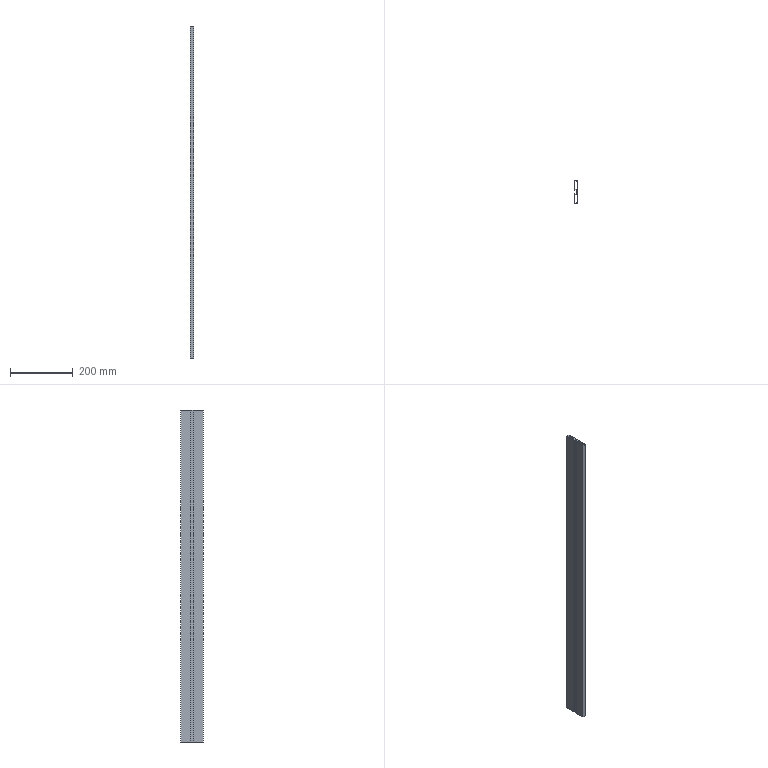Part | 1 solid | 22 faces | box 12 x 73 x 1060 mm | volume 385840 mm3 | plane 22
STEP:
#1=CARTESIAN_POINT('',(-12.,36.5,530.));
#2=VERTEX_POINT('',#1);
#3=CARTESIAN_POINT('',(-12.,4.5,530.));
#4=VERTEX_POINT('',#3);
#5=CARTESIAN_POINT('',(-12.,36.5,530.));
#6=DIRECTION('',(0.,-1.,0.));
#7=VECTOR('',#6,1000.);
#8=LINE('',#5,#7);
#9=EDGE_CURVE('',#2,#4,#8,.T.);
#10=ORIENTED_EDGE('',*,*,#9,.T.);
#11=CARTESIAN_POINT('',(-10.,4.5,530.));
#12=VERTEX_POINT('',#11);
#13=CARTESIAN_POINT('',(-12.,4.5,530.));
#14=DIRECTION('',(1.,0.,0.));
#15=VECTOR('',#14,1000.);
#16=LINE('',#13,#15);
#17=EDGE_CURVE('',#4,#12,#16,.T.);
#18=ORIENTED_EDGE('',*,*,#17,.T.);
#19=CARTESIAN_POINT('',(-10.,6.5,530.));
#20=VERTEX_POINT('',#19);
#21=CARTESIAN_POINT('',(-10.,4.5,530.));
#22=DIRECTION('',(0.,1.,0.));
#23=VECTOR('',#22,1000.);
#24=LINE('',#21,#23);
#25=EDGE_CURVE('',#12,#20,#24,.T.);
#26=ORIENTED_EDGE('',*,*,#25,.T.);
#27=CARTESIAN_POINT('',(-4.,6.5,530.));
#28=VERTEX_POINT('',#27);
#29=CARTESIAN_POINT('',(-10.,6.5,530.));
#30=DIRECTION('',(1.,0.,0.));
#31=VECTOR('',#30,1000.);
#32=LINE('',#29,#31);
#33=EDGE_CURVE('',#20,#28,#32,.T.);
#34=ORIENTED_EDGE('',*,*,#33,.T.);
#35=CARTESIAN_POINT('',(-4.,-6.5,530.));
#36=VERTEX_POINT('',#35);
#37=CARTESIAN_POINT('',(-4.,6.5,530.));
#38=DIRECTION('',(0.,-1.,0.));
#39=VECTOR('',#38,1000.);
#40=LINE('',#37,#39);
#41=EDGE_CURVE('',#28,#36,#40,.T.);
#42=ORIENTED_EDGE('',*,*,#41,.T.);
#43=CARTESIAN_POINT('',(-10.,-6.5,530.));
#44=VERTEX_POINT('',#43);
#45=CARTESIAN_POINT('',(-4.,-6.5,530.));
#46=DIRECTION('',(-1.,0.,0.));
#47=VECTOR('',#46,1000.);
#48=LINE('',#45,#47);
#49=EDGE_CURVE('',#36,#44,#48,.T.);
#50=ORIENTED_EDGE('',*,*,#49,.T.);
#51=CARTESIAN_POINT('',(-10.,-4.5,530.));
#52=VERTEX_POINT('',#51);
#53=CARTESIAN_POINT('',(-10.,-6.5,530.));
#54=DIRECTION('',(0.,1.,0.));
#55=VECTOR('',#54,1000.);
#56=LINE('',#53,#55);
#57=EDGE_CURVE('',#44,#52,#56,.T.);
#58=ORIENTED_EDGE('',*,*,#57,.T.);
#59=CARTESIAN_POINT('',(-12.,-4.5,530.));
#60=VERTEX_POINT('',#59);
#61=CARTESIAN_POINT('',(-10.,-4.5,530.));
#62=DIRECTION('',(-1.,0.,0.));
#63=VECTOR('',#62,1000.);
#64=LINE('',#61,#63);
#65=EDGE_CURVE('',#52,#60,#64,.T.);
#66=ORIENTED_EDGE('',*,*,#65,.T.);
#67=CARTESIAN_POINT('',(-12.,-36.5,530.));
#68=VERTEX_POINT('',#67);
#69=CARTESIAN_POINT('',(-12.,-4.5,530.));
#70=DIRECTION('',(0.,-1.,0.));
#71=VECTOR('',#70,1000.);
#72=LINE('',#69,#71);
#73=EDGE_CURVE('',#60,#68,#72,.T.);
#74=ORIENTED_EDGE('',*,*,#73,.T.);
#75=CARTESIAN_POINT('',(0.,-36.5,530.));
#76=VERTEX_POINT('',#75);
#77=CARTESIAN_POINT('',(-12.,-36.5,530.));
#78=DIRECTION('',(1.,0.,0.));
#79=VECTOR('',#78,1000.);
#80=LINE('',#77,#79);
#81=EDGE_CURVE('',#68,#76,#80,.T.);
#82=ORIENTED_EDGE('',*,*,#81,.T.);
#83=CARTESIAN_POINT('',(0.,36.5,530.));
#84=VERTEX_POINT('',#83);
#85=CARTESIAN_POINT('',(0.,-36.5,530.));
#86=DIRECTION('',(0.,1.,0.));
#87=VECTOR('',#86,1000.);
#88=LINE('',#85,#87);
#89=EDGE_CURVE('',#76,#84,#88,.T.);
#90=ORIENTED_EDGE('',*,*,#89,.T.);
#91=CARTESIAN_POINT('',(0.,36.5,530.));
#92=DIRECTION('',(-1.,0.,0.));
#93=VECTOR('',#92,1000.);
#94=LINE('',#91,#93);
#95=EDGE_CURVE('',#84,#2,#94,.T.);
#96=ORIENTED_EDGE('',*,*,#95,.T.);
#97=EDGE_LOOP('',(#10,#18,#26,#34,#42,#50,#58,#66,#74,#82,#90,#96));
#98=FACE_OUTER_BOUND('',#97,.T.);
#99=CARTESIAN_POINT('',(-10.,-34.5,530.));
#100=VERTEX_POINT('',#99);
#101=CARTESIAN_POINT('',(-2.,-34.5,530.));
#102=VERTEX_POINT('',#101);
#103=CARTESIAN_POINT('',(-2.,-34.5,530.));
#104=DIRECTION('',(1.,0.,0.));
#105=VECTOR('',#104,1000.);
#106=LINE('',#103,#105);
#107=EDGE_CURVE('',#100,#102,#106,.T.);
#108=ORIENTED_EDGE('',*,*,#107,.F.);
#109=CARTESIAN_POINT('',(-10.,-8.5,530.));
#110=VERTEX_POINT('',#109);
#111=CARTESIAN_POINT('',(-10.,-34.5,530.));
#112=DIRECTION('',(0.,-1.,0.));
#113=VECTOR('',#112,1000.);
#114=LINE('',#111,#113);
#115=EDGE_CURVE('',#110,#100,#114,.T.);
#116=ORIENTED_EDGE('',*,*,#115,.F.);
#117=CARTESIAN_POINT('',(-2.,-8.5,530.));
#118=VERTEX_POINT('',#117);
#119=CARTESIAN_POINT('',(-10.,-8.5,530.));
#120=DIRECTION('',(-1.,0.,0.));
#121=VECTOR('',#120,1000.);
#122=LINE('',#119,#121);
#123=EDGE_CURVE('',#118,#110,#122,.T.);
#124=ORIENTED_EDGE('',*,*,#123,.F.);
#125=CARTESIAN_POINT('',(-2.,-8.5,530.));
#126=DIRECTION('',(0.,1.,0.));
#127=VECTOR('',#126,1000.);
#128=LINE('',#125,#127);
#129=EDGE_CURVE('',#102,#118,#128,.T.);
#130=ORIENTED_EDGE('',*,*,#129,.F.);
#131=EDGE_LOOP('',(#108,#116,#124,#130));
#132=FACE_BOUND('',#131,.T.);
#133=CARTESIAN_POINT('',(-10.,34.5,530.));
#134=VERTEX_POINT('',#133);
#135=CARTESIAN_POINT('',(-10.,8.5,530.));
#136=VERTEX_POINT('',#135);
#137=CARTESIAN_POINT('',(-10.,8.5,530.));
#138=DIRECTION('',(0.,-1.,0.));
#139=VECTOR('',#138,1000.);
#140=LINE('',#137,#139);
#141=EDGE_CURVE('',#134,#136,#140,.T.);
#142=ORIENTED_EDGE('',*,*,#141,.F.);
#143=CARTESIAN_POINT('',(-2.,34.5,530.));
#144=VERTEX_POINT('',#143);
#145=CARTESIAN_POINT('',(-10.,34.5,530.));
#146=DIRECTION('',(-1.,0.,0.));
#147=VECTOR('',#146,1000.);
#148=LINE('',#145,#147);
#149=EDGE_CURVE('',#144,#134,#148,.T.);
#150=ORIENTED_EDGE('',*,*,#149,.F.);
#151=CARTESIAN_POINT('',(-2.,8.5,530.));
#152=VERTEX_POINT('',#151);
#153=CARTESIAN_POINT('',(-2.,34.5,530.));
#154=DIRECTION('',(0.,1.,0.));
#155=VECTOR('',#154,1000.);
#156=LINE('',#153,#155);
#157=EDGE_CURVE('',#152,#144,#156,.T.);
#158=ORIENTED_EDGE('',*,*,#157,.F.);
#159=CARTESIAN_POINT('',(-2.,8.5,530.));
#160=DIRECTION('',(1.,0.,0.));
#161=VECTOR('',#160,1000.);
#162=LINE('',#159,#161);
#163=EDGE_CURVE('',#136,#152,#162,.T.);
#164=ORIENTED_EDGE('',*,*,#163,.F.);
#165=EDGE_LOOP('',(#142,#150,#158,#164));
#166=FACE_BOUND('',#165,.T.);
#167=CARTESIAN_POINT('',(0.,0.,530.));
#168=DIRECTION('',(0.,0.,1.));
#169=DIRECTION('',(1.,0.,0.));
#170=AXIS2_PLACEMENT_3D('',#167,#168,#169);
#171=PLANE('',#170);
#172=ADVANCED_FACE('',(#98,#132,#166),#171,.T.);
#173=CARTESIAN_POINT('',(-10.,-8.5,-530.));
#174=VERTEX_POINT('',#173);
#175=CARTESIAN_POINT('',(-10.,-34.5,-530.));
#176=VERTEX_POINT('',#175);
#177=CARTESIAN_POINT('',(-10.,-34.5,-530.));
#178=DIRECTION('',(0.,-1.,0.));
#179=VECTOR('',#178,1000.);
#180=LINE('',#177,#179);
#181=EDGE_CURVE('',#174,#176,#180,.T.);
#182=ORIENTED_EDGE('',*,*,#181,.T.);
#183=CARTESIAN_POINT('',(-2.,-34.5,-530.));
#184=VERTEX_POINT('',#183);
#185=CARTESIAN_POINT('',(-2.,-34.5,-530.));
#186=DIRECTION('',(1.,0.,0.));
#187=VECTOR('',#186,1000.);
#188=LINE('',#185,#187);
#189=EDGE_CURVE('',#176,#184,#188,.T.);
#190=ORIENTED_EDGE('',*,*,#189,.T.);
#191=CARTESIAN_POINT('',(-2.,-8.5,-530.));
#192=VERTEX_POINT('',#191);
#193=CARTESIAN_POINT('',(-2.,-8.5,-530.));
#194=DIRECTION('',(0.,1.,0.));
#195=VECTOR('',#194,1000.);
#196=LINE('',#193,#195);
#197=EDGE_CURVE('',#184,#192,#196,.T.);
#198=ORIENTED_EDGE('',*,*,#197,.T.);
#199=CARTESIAN_POINT('',(-10.,-8.5,-530.));
#200=DIRECTION('',(-1.,0.,0.));
#201=VECTOR('',#200,1000.);
#202=LINE('',#199,#201);
#203=EDGE_CURVE('',#192,#174,#202,.T.);
#204=ORIENTED_EDGE('',*,*,#203,.T.);
#205=EDGE_LOOP('',(#182,#190,#198,#204));
#206=FACE_BOUND('',#205,.T.);
#207=CARTESIAN_POINT('',(-12.,36.5,-530.));
#208=VERTEX_POINT('',#207);
#209=CARTESIAN_POINT('',(-12.,4.5,-530.));
#210=VERTEX_POINT('',#209);
#211=CARTESIAN_POINT('',(-12.,36.5,-530.));
#212=DIRECTION('',(0.,-1.,0.));
#213=VECTOR('',#212,1000.);
#214=LINE('',#211,#213);
#215=EDGE_CURVE('',#208,#210,#214,.T.);
#216=ORIENTED_EDGE('',*,*,#215,.F.);
#217=CARTESIAN_POINT('',(0.,36.5,-530.));
#218=VERTEX_POINT('',#217);
#219=CARTESIAN_POINT('',(0.,36.5,-530.));
#220=DIRECTION('',(-1.,0.,0.));
#221=VECTOR('',#220,1000.);
#222=LINE('',#219,#221);
#223=EDGE_CURVE('',#218,#208,#222,.T.);
#224=ORIENTED_EDGE('',*,*,#223,.F.);
#225=CARTESIAN_POINT('',(0.,-36.5,-530.));
#226=VERTEX_POINT('',#225);
#227=CARTESIAN_POINT('',(0.,-36.5,-530.));
#228=DIRECTION('',(0.,1.,0.));
#229=VECTOR('',#228,1000.);
#230=LINE('',#227,#229);
#231=EDGE_CURVE('',#226,#218,#230,.T.);
#232=ORIENTED_EDGE('',*,*,#231,.F.);
#233=CARTESIAN_POINT('',(-12.,-36.5,-530.));
#234=VERTEX_POINT('',#233);
#235=CARTESIAN_POINT('',(-12.,-36.5,-530.));
#236=DIRECTION('',(1.,0.,0.));
#237=VECTOR('',#236,1000.);
#238=LINE('',#235,#237);
#239=EDGE_CURVE('',#234,#226,#238,.T.);
#240=ORIENTED_EDGE('',*,*,#239,.F.);
#241=CARTESIAN_POINT('',(-12.,-4.5,-530.));
#242=VERTEX_POINT('',#241);
#243=CARTESIAN_POINT('',(-12.,-4.5,-530.));
#244=DIRECTION('',(0.,-1.,0.));
#245=VECTOR('',#244,1000.);
#246=LINE('',#243,#245);
#247=EDGE_CURVE('',#242,#234,#246,.T.);
#248=ORIENTED_EDGE('',*,*,#247,.F.);
#249=CARTESIAN_POINT('',(-10.,-4.5,-530.));
#250=VERTEX_POINT('',#249);
#251=CARTESIAN_POINT('',(-10.,-4.5,-530.));
#252=DIRECTION('',(-1.,0.,0.));
#253=VECTOR('',#252,1000.);
#254=LINE('',#251,#253);
#255=EDGE_CURVE('',#250,#242,#254,.T.);
#256=ORIENTED_EDGE('',*,*,#255,.F.);
#257=CARTESIAN_POINT('',(-10.,-6.5,-530.));
#258=VERTEX_POINT('',#257);
#259=CARTESIAN_POINT('',(-10.,-6.5,-530.));
#260=DIRECTION('',(0.,1.,0.));
#261=VECTOR('',#260,1000.);
#262=LINE('',#259,#261);
#263=EDGE_CURVE('',#258,#250,#262,.T.);
#264=ORIENTED_EDGE('',*,*,#263,.F.);
#265=CARTESIAN_POINT('',(-4.,-6.5,-530.));
#266=VERTEX_POINT('',#265);
#267=CARTESIAN_POINT('',(-4.,-6.5,-530.));
#268=DIRECTION('',(-1.,0.,0.));
#269=VECTOR('',#268,1000.);
#270=LINE('',#267,#269);
#271=EDGE_CURVE('',#266,#258,#270,.T.);
#272=ORIENTED_EDGE('',*,*,#271,.F.);
#273=CARTESIAN_POINT('',(-4.,6.5,-530.));
#274=VERTEX_POINT('',#273);
#275=CARTESIAN_POINT('',(-4.,6.5,-530.));
#276=DIRECTION('',(0.,-1.,0.));
#277=VECTOR('',#276,1000.);
#278=LINE('',#275,#277);
#279=EDGE_CURVE('',#274,#266,#278,.T.);
#280=ORIENTED_EDGE('',*,*,#279,.F.);
#281=CARTESIAN_POINT('',(-10.,6.5,-530.));
#282=VERTEX_POINT('',#281);
#283=CARTESIAN_POINT('',(-10.,6.5,-530.));
#284=DIRECTION('',(1.,0.,0.));
#285=VECTOR('',#284,1000.);
#286=LINE('',#283,#285);
#287=EDGE_CURVE('',#282,#274,#286,.T.);
#288=ORIENTED_EDGE('',*,*,#287,.F.);
#289=CARTESIAN_POINT('',(-10.,4.5,-530.));
#290=VERTEX_POINT('',#289);
#291=CARTESIAN_POINT('',(-10.,4.5,-530.));
#292=DIRECTION('',(0.,1.,0.));
#293=VECTOR('',#292,1000.);
#294=LINE('',#291,#293);
#295=EDGE_CURVE('',#290,#282,#294,.T.);
#296=ORIENTED_EDGE('',*,*,#295,.F.);
#297=CARTESIAN_POINT('',(-12.,4.5,-530.));
#298=DIRECTION('',(1.,0.,0.));
#299=VECTOR('',#298,1000.);
#300=LINE('',#297,#299);
#301=EDGE_CURVE('',#210,#290,#300,.T.);
#302=ORIENTED_EDGE('',*,*,#301,.F.);
#303=EDGE_LOOP('',(#216,#224,#232,#240,#248,#256,#264,#272,#280,#288,#296,#302));
#304=FACE_OUTER_BOUND('',#303,.T.);
#305=CARTESIAN_POINT('',(-2.,34.5,-530.));
#306=VERTEX_POINT('',#305);
#307=CARTESIAN_POINT('',(-10.,34.5,-530.));
#308=VERTEX_POINT('',#307);
#309=CARTESIAN_POINT('',(-10.,34.5,-530.));
#310=DIRECTION('',(-1.,0.,0.));
#311=VECTOR('',#310,1000.);
#312=LINE('',#309,#311);
#313=EDGE_CURVE('',#306,#308,#312,.T.);
#314=ORIENTED_EDGE('',*,*,#313,.T.);
#315=CARTESIAN_POINT('',(-10.,8.5,-530.));
#316=VERTEX_POINT('',#315);
#317=CARTESIAN_POINT('',(-10.,8.5,-530.));
#318=DIRECTION('',(0.,-1.,0.));
#319=VECTOR('',#318,1000.);
#320=LINE('',#317,#319);
#321=EDGE_CURVE('',#308,#316,#320,.T.);
#322=ORIENTED_EDGE('',*,*,#321,.T.);
#323=CARTESIAN_POINT('',(-2.,8.5,-530.));
#324=VERTEX_POINT('',#323);
#325=CARTESIAN_POINT('',(-2.,8.5,-530.));
#326=DIRECTION('',(1.,0.,0.));
#327=VECTOR('',#326,1000.);
#328=LINE('',#325,#327);
#329=EDGE_CURVE('',#316,#324,#328,.T.);
#330=ORIENTED_EDGE('',*,*,#329,.T.);
#331=CARTESIAN_POINT('',(-2.,34.5,-530.));
#332=DIRECTION('',(0.,1.,0.));
#333=VECTOR('',#332,1000.);
#334=LINE('',#331,#333);
#335=EDGE_CURVE('',#324,#306,#334,.T.);
#336=ORIENTED_EDGE('',*,*,#335,.T.);
#337=EDGE_LOOP('',(#314,#322,#330,#336));
#338=FACE_BOUND('',#337,.T.);
#339=CARTESIAN_POINT('',(0.,0.,-530.));
#340=DIRECTION('',(0.,0.,1.));
#341=DIRECTION('',(1.,0.,0.));
#342=AXIS2_PLACEMENT_3D('',#339,#340,#341);
#343=PLANE('',#342);
#344=ADVANCED_FACE('',(#206,#304,#338),#343,.F.);
#345=ORIENTED_EDGE('',*,*,#215,.T.);
#346=CARTESIAN_POINT('',(-12.,4.5,530.));
#347=DIRECTION('',(0.,0.,-1.));
#348=VECTOR('',#347,1000.);
#349=LINE('',#346,#348);
#350=EDGE_CURVE('',#4,#210,#349,.T.);
#351=ORIENTED_EDGE('',*,*,#350,.F.);
#352=ORIENTED_EDGE('',*,*,#9,.F.);
#353=CARTESIAN_POINT('',(-12.,36.5,530.));
#354=DIRECTION('',(0.,0.,-1.));
#355=VECTOR('',#354,1000.);
#356=LINE('',#353,#355);
#357=EDGE_CURVE('',#2,#208,#356,.T.);
#358=ORIENTED_EDGE('',*,*,#357,.T.);
#359=EDGE_LOOP('',(#345,#351,#352,#358));
#360=FACE_OUTER_BOUND('',#359,.T.);
#361=CARTESIAN_POINT('',(-12.,36.5,530.));
#362=DIRECTION('',(1.,0.,0.));
#363=DIRECTION('',(0.,0.,-1.));
#364=AXIS2_PLACEMENT_3D('',#361,#362,#363);
#365=PLANE('',#364);
#366=ADVANCED_FACE('',(#360),#365,.F.);
#367=ORIENTED_EDGE('',*,*,#301,.T.);
#368=CARTESIAN_POINT('',(-10.,4.5,530.));
#369=DIRECTION('',(0.,0.,-1.));
#370=VECTOR('',#369,1000.);
#371=LINE('',#368,#370);
#372=EDGE_CURVE('',#12,#290,#371,.T.);
#373=ORIENTED_EDGE('',*,*,#372,.F.);
#374=ORIENTED_EDGE('',*,*,#17,.F.);
#375=ORIENTED_EDGE('',*,*,#350,.T.);
#376=EDGE_LOOP('',(#367,#373,#374,#375));
#377=FACE_OUTER_BOUND('',#376,.T.);
#378=CARTESIAN_POINT('',(-12.,4.5,530.));
#379=DIRECTION('',(0.,1.,0.));
#380=DIRECTION('',(0.,0.,1.));
#381=AXIS2_PLACEMENT_3D('',#378,#379,#380);
#382=PLANE('',#381);
#383=ADVANCED_FACE('',(#377),#382,.F.);
#384=ORIENTED_EDGE('',*,*,#295,.T.);
#385=CARTESIAN_POINT('',(-10.,6.5,530.));
#386=DIRECTION('',(0.,0.,-1.));
#387=VECTOR('',#386,1000.);
#388=LINE('',#385,#387);
#389=EDGE_CURVE('',#20,#282,#388,.T.);
#390=ORIENTED_EDGE('',*,*,#389,.F.);
#391=ORIENTED_EDGE('',*,*,#25,.F.);
#392=ORIENTED_EDGE('',*,*,#372,.T.);
#393=EDGE_LOOP('',(#384,#390,#391,#392));
#394=FACE_OUTER_BOUND('',#393,.T.);
#395=CARTESIAN_POINT('',(-10.,4.5,530.));
#396=DIRECTION('',(-1.,0.,0.));
#397=DIRECTION('',(0.,0.,1.));
#398=AXIS2_PLACEMENT_3D('',#395,#396,#397);
#399=PLANE('',#398);
#400=ADVANCED_FACE('',(#394),#399,.F.);
#401=ORIENTED_EDGE('',*,*,#287,.T.);
#402=CARTESIAN_POINT('',(-4.,6.5,530.));
#403=DIRECTION('',(0.,0.,-1.));
#404=VECTOR('',#403,1000.);
#405=LINE('',#402,#404);
#406=EDGE_CURVE('',#28,#274,#405,.T.);
#407=ORIENTED_EDGE('',*,*,#406,.F.);
#408=ORIENTED_EDGE('',*,*,#33,.F.);
#409=ORIENTED_EDGE('',*,*,#389,.T.);
#410=EDGE_LOOP('',(#401,#407,#408,#409));
#411=FACE_OUTER_BOUND('',#410,.T.);
#412=CARTESIAN_POINT('',(-10.,6.5,530.));
#413=DIRECTION('',(0.,1.,0.));
#414=DIRECTION('',(0.,0.,1.));
#415=AXIS2_PLACEMENT_3D('',#412,#413,#414);
#416=PLANE('',#415);
#417=ADVANCED_FACE('',(#411),#416,.F.);
#418=ORIENTED_EDGE('',*,*,#279,.T.);
#419=CARTESIAN_POINT('',(-4.,-6.5,530.));
#420=DIRECTION('',(0.,0.,-1.));
#421=VECTOR('',#420,1000.);
#422=LINE('',#419,#421);
#423=EDGE_CURVE('',#36,#266,#422,.T.);
#424=ORIENTED_EDGE('',*,*,#423,.F.);
#425=ORIENTED_EDGE('',*,*,#41,.F.);
#426=ORIENTED_EDGE('',*,*,#406,.T.);
#427=EDGE_LOOP('',(#418,#424,#425,#426));
#428=FACE_OUTER_BOUND('',#427,.T.);
#429=CARTESIAN_POINT('',(-4.,6.5,530.));
#430=DIRECTION('',(1.,0.,0.));
#431=DIRECTION('',(0.,0.,-1.));
#432=AXIS2_PLACEMENT_3D('',#429,#430,#431);
#433=PLANE('',#432);
#434=ADVANCED_FACE('',(#428),#433,.F.);
#435=ORIENTED_EDGE('',*,*,#271,.T.);
#436=CARTESIAN_POINT('',(-10.,-6.5,530.));
#437=DIRECTION('',(0.,0.,-1.));
#438=VECTOR('',#437,1000.);
#439=LINE('',#436,#438);
#440=EDGE_CURVE('',#44,#258,#439,.T.);
#441=ORIENTED_EDGE('',*,*,#440,.F.);
#442=ORIENTED_EDGE('',*,*,#49,.F.);
#443=ORIENTED_EDGE('',*,*,#423,.T.);
#444=EDGE_LOOP('',(#435,#441,#442,#443));
#445=FACE_OUTER_BOUND('',#444,.T.);
#446=CARTESIAN_POINT('',(-4.,-6.5,530.));
#447=DIRECTION('',(0.,-1.,0.));
#448=DIRECTION('',(0.,0.,-1.));
#449=AXIS2_PLACEMENT_3D('',#446,#447,#448);
#450=PLANE('',#449);
#451=ADVANCED_FACE('',(#445),#450,.F.);
#452=ORIENTED_EDGE('',*,*,#263,.T.);
#453=CARTESIAN_POINT('',(-10.,-4.5,530.));
#454=DIRECTION('',(0.,0.,-1.));
#455=VECTOR('',#454,1000.);
#456=LINE('',#453,#455);
#457=EDGE_CURVE('',#52,#250,#456,.T.);
#458=ORIENTED_EDGE('',*,*,#457,.F.);
#459=ORIENTED_EDGE('',*,*,#57,.F.);
#460=ORIENTED_EDGE('',*,*,#440,.T.);
#461=EDGE_LOOP('',(#452,#458,#459,#460));
#462=FACE_OUTER_BOUND('',#461,.T.);
#463=CARTESIAN_POINT('',(-10.,-6.5,530.));
#464=DIRECTION('',(-1.,0.,0.));
#465=DIRECTION('',(0.,0.,1.));
#466=AXIS2_PLACEMENT_3D('',#463,#464,#465);
#467=PLANE('',#466);
#468=ADVANCED_FACE('',(#462),#467,.F.);
#469=ORIENTED_EDGE('',*,*,#255,.T.);
#470=CARTESIAN_POINT('',(-12.,-4.5,530.));
#471=DIRECTION('',(0.,0.,-1.));
#472=VECTOR('',#471,1000.);
#473=LINE('',#470,#472);
#474=EDGE_CURVE('',#60,#242,#473,.T.);
#475=ORIENTED_EDGE('',*,*,#474,.F.);
#476=ORIENTED_EDGE('',*,*,#65,.F.);
#477=ORIENTED_EDGE('',*,*,#457,.T.);
#478=EDGE_LOOP('',(#469,#475,#476,#477));
#479=FACE_OUTER_BOUND('',#478,.T.);
#480=CARTESIAN_POINT('',(-10.,-4.5,530.));
#481=DIRECTION('',(0.,-1.,0.));
#482=DIRECTION('',(0.,0.,-1.));
#483=AXIS2_PLACEMENT_3D('',#480,#481,#482);
#484=PLANE('',#483);
#485=ADVANCED_FACE('',(#479),#484,.F.);
#486=ORIENTED_EDGE('',*,*,#247,.T.);
#487=CARTESIAN_POINT('',(-12.,-36.5,530.));
#488=DIRECTION('',(0.,0.,-1.));
#489=VECTOR('',#488,1000.);
#490=LINE('',#487,#489);
#491=EDGE_CURVE('',#68,#234,#490,.T.);
#492=ORIENTED_EDGE('',*,*,#491,.F.);
#493=ORIENTED_EDGE('',*,*,#73,.F.);
#494=ORIENTED_EDGE('',*,*,#474,.T.);
#495=EDGE_LOOP('',(#486,#492,#493,#494));
#496=FACE_OUTER_BOUND('',#495,.T.);
#497=CARTESIAN_POINT('',(-12.,-4.5,530.));
#498=DIRECTION('',(1.,0.,0.));
#499=DIRECTION('',(0.,0.,-1.));
#500=AXIS2_PLACEMENT_3D('',#497,#498,#499);
#501=PLANE('',#500);
#502=ADVANCED_FACE('',(#496),#501,.F.);
#503=ORIENTED_EDGE('',*,*,#239,.T.);
#504=CARTESIAN_POINT('',(0.,-36.5,530.));
#505=DIRECTION('',(0.,0.,-1.));
#506=VECTOR('',#505,1000.);
#507=LINE('',#504,#506);
#508=EDGE_CURVE('',#76,#226,#507,.T.);
#509=ORIENTED_EDGE('',*,*,#508,.F.);
#510=ORIENTED_EDGE('',*,*,#81,.F.);
#511=ORIENTED_EDGE('',*,*,#491,.T.);
#512=EDGE_LOOP('',(#503,#509,#510,#511));
#513=FACE_OUTER_BOUND('',#512,.T.);
#514=CARTESIAN_POINT('',(-12.,-36.5,530.));
#515=DIRECTION('',(0.,1.,0.));
#516=DIRECTION('',(0.,0.,1.));
#517=AXIS2_PLACEMENT_3D('',#514,#515,#516);
#518=PLANE('',#517);
#519=ADVANCED_FACE('',(#513),#518,.F.);
#520=ORIENTED_EDGE('',*,*,#231,.T.);
#521=CARTESIAN_POINT('',(0.,36.5,530.));
#522=DIRECTION('',(0.,0.,-1.));
#523=VECTOR('',#522,1000.);
#524=LINE('',#521,#523);
#525=EDGE_CURVE('',#84,#218,#524,.T.);
#526=ORIENTED_EDGE('',*,*,#525,.F.);
#527=ORIENTED_EDGE('',*,*,#89,.F.);
#528=ORIENTED_EDGE('',*,*,#508,.T.);
#529=EDGE_LOOP('',(#520,#526,#527,#528));
#530=FACE_OUTER_BOUND('',#529,.T.);
#531=CARTESIAN_POINT('',(0.,-36.5,530.));
#532=DIRECTION('',(-1.,0.,0.));
#533=DIRECTION('',(0.,0.,1.));
#534=AXIS2_PLACEMENT_3D('',#531,#532,#533);
#535=PLANE('',#534);
#536=ADVANCED_FACE('',(#530),#535,.F.);
#537=ORIENTED_EDGE('',*,*,#223,.T.);
#538=ORIENTED_EDGE('',*,*,#357,.F.);
#539=ORIENTED_EDGE('',*,*,#95,.F.);
#540=ORIENTED_EDGE('',*,*,#525,.T.);
#541=EDGE_LOOP('',(#537,#538,#539,#540));
#542=FACE_OUTER_BOUND('',#541,.T.);
#543=CARTESIAN_POINT('',(0.,36.5,530.));
#544=DIRECTION('',(0.,-1.,0.));
#545=DIRECTION('',(0.,0.,-1.));
#546=AXIS2_PLACEMENT_3D('',#543,#544,#545);
#547=PLANE('',#546);
#548=ADVANCED_FACE('',(#542),#547,.F.);
#549=ORIENTED_EDGE('',*,*,#181,.F.);
#550=CARTESIAN_POINT('',(-10.,-8.5,530.));
#551=DIRECTION('',(0.,0.,-1.));
#552=VECTOR('',#551,1000.);
#553=LINE('',#550,#552);
#554=EDGE_CURVE('',#110,#174,#553,.T.);
#555=ORIENTED_EDGE('',*,*,#554,.F.);
#556=ORIENTED_EDGE('',*,*,#115,.T.);
#557=CARTESIAN_POINT('',(-10.,-34.5,530.));
#558=DIRECTION('',(0.,0.,-1.));
#559=VECTOR('',#558,1000.);
#560=LINE('',#557,#559);
#561=EDGE_CURVE('',#100,#176,#560,.T.);
#562=ORIENTED_EDGE('',*,*,#561,.T.);
#563=EDGE_LOOP('',(#549,#555,#556,#562));
#564=FACE_OUTER_BOUND('',#563,.T.);
#565=CARTESIAN_POINT('',(-10.,-34.5,530.));
#566=DIRECTION('',(1.,0.,0.));
#567=DIRECTION('',(0.,0.,-1.));
#568=AXIS2_PLACEMENT_3D('',#565,#566,#567);
#569=PLANE('',#568);
#570=ADVANCED_FACE('',(#564),#569,.T.);
#571=ORIENTED_EDGE('',*,*,#189,.F.);
#572=ORIENTED_EDGE('',*,*,#561,.F.);
#573=ORIENTED_EDGE('',*,*,#107,.T.);
#574=CARTESIAN_POINT('',(-2.,-34.5,530.));
#575=DIRECTION('',(0.,0.,-1.));
#576=VECTOR('',#575,1000.);
#577=LINE('',#574,#576);
#578=EDGE_CURVE('',#102,#184,#577,.T.);
#579=ORIENTED_EDGE('',*,*,#578,.T.);
#580=EDGE_LOOP('',(#571,#572,#573,#579));
#581=FACE_OUTER_BOUND('',#580,.T.);
#582=CARTESIAN_POINT('',(-2.,-34.5,530.));
#583=DIRECTION('',(0.,1.,0.));
#584=DIRECTION('',(0.,0.,1.));
#585=AXIS2_PLACEMENT_3D('',#582,#583,#584);
#586=PLANE('',#585);
#587=ADVANCED_FACE('',(#581),#586,.T.);
#588=ORIENTED_EDGE('',*,*,#197,.F.);
#589=ORIENTED_EDGE('',*,*,#578,.F.);
#590=ORIENTED_EDGE('',*,*,#129,.T.);
#591=CARTESIAN_POINT('',(-2.,-8.5,530.));
#592=DIRECTION('',(0.,0.,-1.));
#593=VECTOR('',#592,1000.);
#594=LINE('',#591,#593);
#595=EDGE_CURVE('',#118,#192,#594,.T.);
#596=ORIENTED_EDGE('',*,*,#595,.T.);
#597=EDGE_LOOP('',(#588,#589,#590,#596));
#598=FACE_OUTER_BOUND('',#597,.T.);
#599=CARTESIAN_POINT('',(-2.,-8.5,530.));
#600=DIRECTION('',(-1.,0.,0.));
#601=DIRECTION('',(0.,0.,1.));
#602=AXIS2_PLACEMENT_3D('',#599,#600,#601);
#603=PLANE('',#602);
#604=ADVANCED_FACE('',(#598),#603,.T.);
#605=ORIENTED_EDGE('',*,*,#203,.F.);
#606=ORIENTED_EDGE('',*,*,#595,.F.);
#607=ORIENTED_EDGE('',*,*,#123,.T.);
#608=ORIENTED_EDGE('',*,*,#554,.T.);
#609=EDGE_LOOP('',(#605,#606,#607,#608));
#610=FACE_OUTER_BOUND('',#609,.T.);
#611=CARTESIAN_POINT('',(-10.,-8.5,530.));
#612=DIRECTION('',(0.,-1.,0.));
#613=DIRECTION('',(0.,0.,-1.));
#614=AXIS2_PLACEMENT_3D('',#611,#612,#613);
#615=PLANE('',#614);
#616=ADVANCED_FACE('',(#610),#615,.T.);
#617=ORIENTED_EDGE('',*,*,#313,.F.);
#618=CARTESIAN_POINT('',(-2.,34.5,530.));
#619=DIRECTION('',(0.,0.,-1.));
#620=VECTOR('',#619,1000.);
#621=LINE('',#618,#620);
#622=EDGE_CURVE('',#144,#306,#621,.T.);
#623=ORIENTED_EDGE('',*,*,#622,.F.);
#624=ORIENTED_EDGE('',*,*,#149,.T.);
#625=CARTESIAN_POINT('',(-10.,34.5,530.));
#626=DIRECTION('',(0.,0.,-1.));
#627=VECTOR('',#626,1000.);
#628=LINE('',#625,#627);
#629=EDGE_CURVE('',#134,#308,#628,.T.);
#630=ORIENTED_EDGE('',*,*,#629,.T.);
#631=EDGE_LOOP('',(#617,#623,#624,#630));
#632=FACE_OUTER_BOUND('',#631,.T.);
#633=CARTESIAN_POINT('',(-10.,34.5,530.));
#634=DIRECTION('',(0.,-1.,0.));
#635=DIRECTION('',(0.,0.,-1.));
#636=AXIS2_PLACEMENT_3D('',#633,#634,#635);
#637=PLANE('',#636);
#638=ADVANCED_FACE('',(#632),#637,.T.);
#639=ORIENTED_EDGE('',*,*,#321,.F.);
#640=ORIENTED_EDGE('',*,*,#629,.F.);
#641=ORIENTED_EDGE('',*,*,#141,.T.);
#642=CARTESIAN_POINT('',(-10.,8.5,530.));
#643=DIRECTION('',(0.,0.,-1.));
#644=VECTOR('',#643,1000.);
#645=LINE('',#642,#644);
#646=EDGE_CURVE('',#136,#316,#645,.T.);
#647=ORIENTED_EDGE('',*,*,#646,.T.);
#648=EDGE_LOOP('',(#639,#640,#641,#647));
#649=FACE_OUTER_BOUND('',#648,.T.);
#650=CARTESIAN_POINT('',(-10.,8.5,530.));
#651=DIRECTION('',(1.,0.,0.));
#652=DIRECTION('',(0.,0.,-1.));
#653=AXIS2_PLACEMENT_3D('',#650,#651,#652);
#654=PLANE('',#653);
#655=ADVANCED_FACE('',(#649),#654,.T.);
#656=ORIENTED_EDGE('',*,*,#329,.F.);
#657=ORIENTED_EDGE('',*,*,#646,.F.);
#658=ORIENTED_EDGE('',*,*,#163,.T.);
#659=CARTESIAN_POINT('',(-2.,8.5,530.));
#660=DIRECTION('',(0.,0.,-1.));
#661=VECTOR('',#660,1000.);
#662=LINE('',#659,#661);
#663=EDGE_CURVE('',#152,#324,#662,.T.);
#664=ORIENTED_EDGE('',*,*,#663,.T.);
#665=EDGE_LOOP('',(#656,#657,#658,#664));
#666=FACE_OUTER_BOUND('',#665,.T.);
#667=CARTESIAN_POINT('',(-2.,8.5,530.));
#668=DIRECTION('',(0.,1.,0.));
#669=DIRECTION('',(0.,0.,1.));
#670=AXIS2_PLACEMENT_3D('',#667,#668,#669);
#671=PLANE('',#670);
#672=ADVANCED_FACE('',(#666),#671,.T.);
#673=ORIENTED_EDGE('',*,*,#335,.F.);
#674=ORIENTED_EDGE('',*,*,#663,.F.);
#675=ORIENTED_EDGE('',*,*,#157,.T.);
#676=ORIENTED_EDGE('',*,*,#622,.T.);
#677=EDGE_LOOP('',(#673,#674,#675,#676));
#678=FACE_OUTER_BOUND('',#677,.T.);
#679=CARTESIAN_POINT('',(-2.,34.5,530.));
#680=DIRECTION('',(-1.,0.,0.));
#681=DIRECTION('',(0.,0.,1.));
#682=AXIS2_PLACEMENT_3D('',#679,#680,#681);
#683=PLANE('',#682);
#684=ADVANCED_FACE('',(#678),#683,.T.);
#685=CLOSED_SHELL('',(#172,#344,#366,#383,#400,#417,#434,#451,#468,#485,#502,#519,#536,#548,#570,#587,#604,#616,#638,#655,#672,#684));
#686=MANIFOLD_SOLID_BREP('',#685);
#687=CARTESIAN_POINT('',(0.,0.,0.));
#688=DIRECTION('',(0.,0.,1.));
#689=DIRECTION('',(1.,0.,0.));
#690=AXIS2_PLACEMENT_3D('',#687,#688,#689);
#691=(LENGTH_UNIT()NAMED_UNIT(*)SI_UNIT(.MILLI.,.METRE.));
#692=UNCERTAINTY_MEASURE_WITH_UNIT(LENGTH_MEASURE(0.00001),#691,'','');
#693=(NAMED_UNIT(*)PLANE_ANGLE_UNIT()SI_UNIT($,.RADIAN.));
#694=(NAMED_UNIT(*)SI_UNIT($,.STERADIAN.)SOLID_ANGLE_UNIT());
#695=(GEOMETRIC_REPRESENTATION_CONTEXT(3)GLOBAL_UNCERTAINTY_ASSIGNED_CONTEXT((#692))GLOBAL_UNIT_ASSIGNED_CONTEXT((#691,#693,#694))REPRESENTATION_CONTEXT('',''));
#696=ADVANCED_BREP_SHAPE_REPRESENTATION('',(#686,#690),#695);